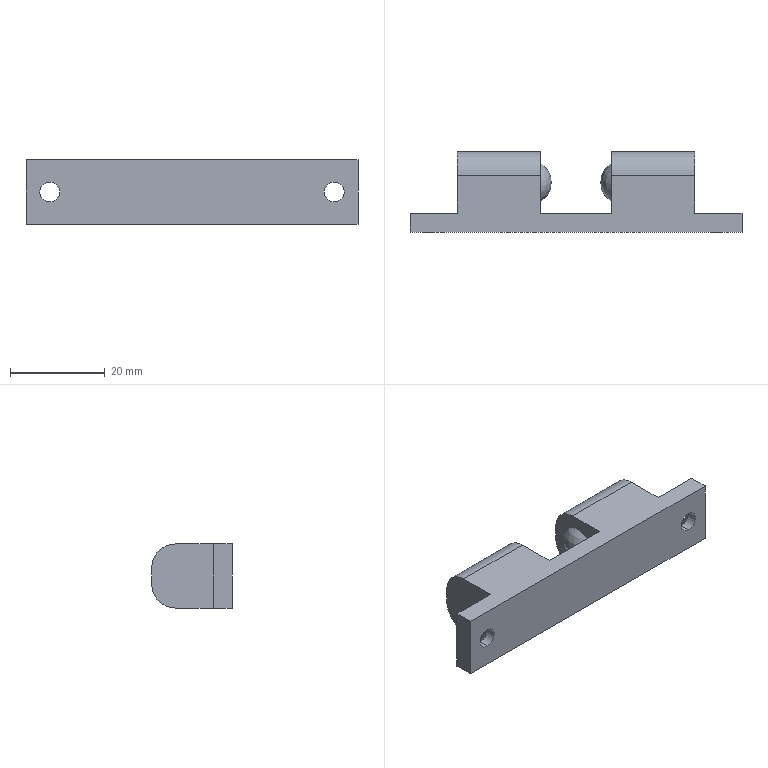Part | STEP file | Ball catch 1 | 1 solid | 30 faces | box 70 x 17 x 13.5 mm | volume 9503 mm3 | plane 14 | cylinder 8 | cone 4 | sphere 4 | commonest cylinder face diameters 4.2 x4 10 x4